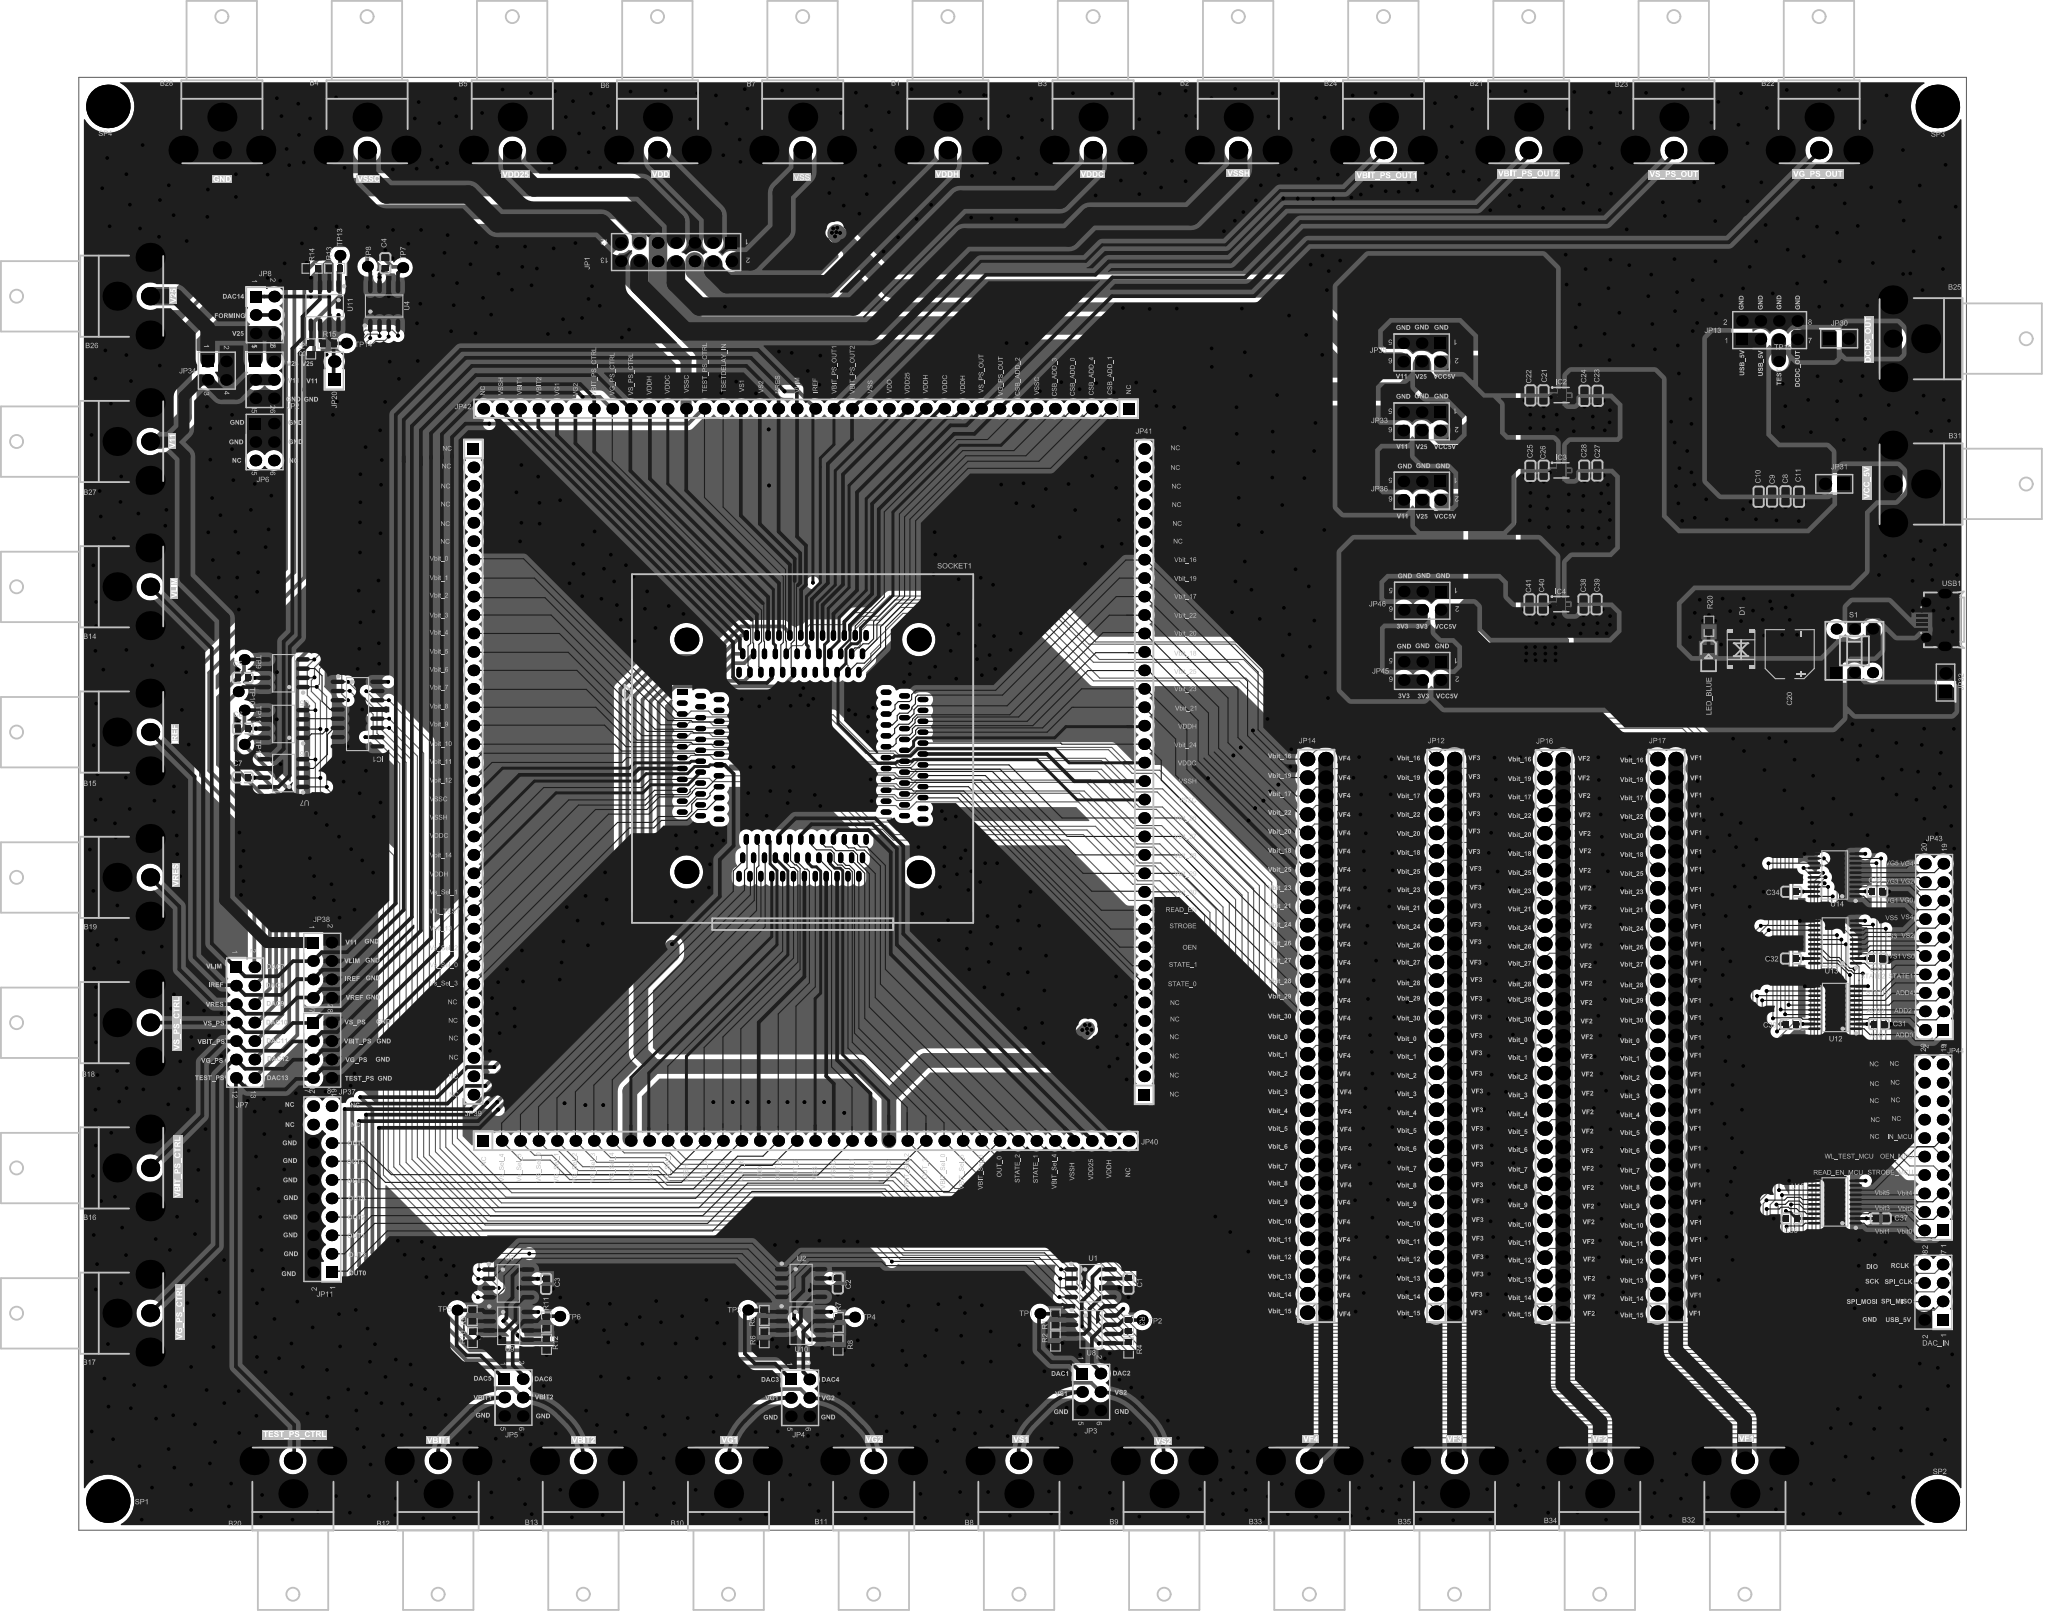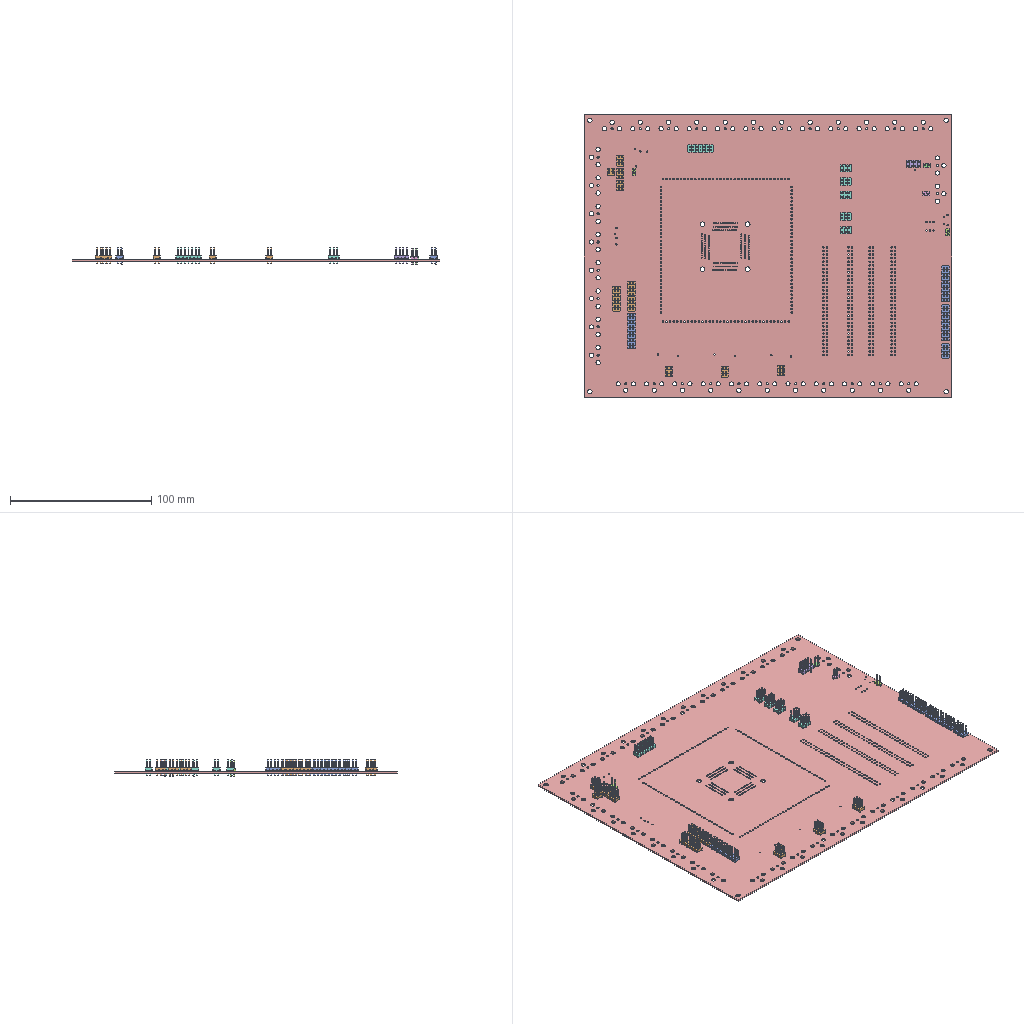Circuit board layout | Altium Designer | box 260 x 200 x 12.2 mm
Layer stack:
# Altium Designer layer stack of  (unit mm; dielectric type: 0 none, 1 core, 2 prepreg, 3 surface material)
index,name,kind,layer,copper_thickness_mm,dielectric_type,dielectric_thickness_mm,dielectric_material,dielectric_constant
0,Top Paste,other,,,,,,
1,Top Overlay,other,,,,,,
2,Top Solder,dielectric,,,3,0.0102,Solder Resist,3.5
3,Top Layer,copper,Top Layer,0.0356,,,,
4,Dielectric1,dielectric,,,1,0.32,FR-4,4.8
5,GND,copper,GND,0.0356,,,,
6,Dielectric3,dielectric,,,2,0.32,FR-4,4.8
7,POWER,copper,POWER,0.0356,,,,
8,Dielectric2,dielectric,,,1,0.32,FR-4,4.8
9,Bottom Layer,copper,Bottom Layer,0.0356,,,,
10,Bottom Solder,dielectric,,,3,0.0102,Solder Resist,3.5
11,Bottom Overlay,other,,,,,,
12,Bottom Paste,other,,,,,,
# drill layer pairs: low layer,high layer
drill_pair,Top Layer,Bottom Layer
Part placement:
Designator,Comment,Layer,Footprint,Center-X(mm),Center-Y(mm),Rotation
U15,TXS0108E,TopLayer,TSSOP-20_L6.5-W4.4-P0.65-LS6.4-BL,241.884,45.187,180
U14,TXS0108E,TopLayer,TSSOP-20_L6.5-W4.4-P0.65-LS6.4-BL,241.859,90.196,180
U13,TXS0108E,TopLayer,TSSOP-20_L6.5-W4.4-P0.65-LS6.4-BL,241.91,80.975,180
U12,TXS0108E,TopLayer,TSSOP-20_L6.5-W4.4-P0.65-LS6.4-BL,241.935,71.958,180
C37,100nF,TopLayer,0603C,248.209,42.926,360
C36,100nF,TopLayer,0603C,235.915,42.901,360
C35,100nF,TopLayer,0603C,247.726,87.91,360
C34,100nF,TopLayer,0603C,235.89,87.884,360
C33,100nF,TopLayer,0603C,247.726,78.689,360
C32,100nF,TopLayer,0603C,235.839,78.689,360
C31,100nF,TopLayer,0603C,247.955,69.672,360
C30,100nF,TopLayer,0603C,235.788,69.672,360
C20,100uF/25V,TopLayer,EC-D6.3x7.7,235.661,120.599,90
DAC_IN,DAC_IN,TopLayer,HDR2.54-LI-2x4P,255.448,32.766,90
U11,LM358,TopLayer,SO-8,33.866,168.564,270
U10,LM358,TopLayer,SO-8,99.469,28.16,360
U9,LM358,TopLayer,SO-8,59.21,28.135,360
U8,LM358,TopLayer,SO-8,139.424,27.652,360
U7,LTC1446,TopLayer,SO-8,28.208,104.228,180
U6,LTC1446,TopLayer,SO-8,28.208,110.984,180
U5,LTC1446,TopLayer,SO-8,28.208,117.969,180
U4,LTC1446,TopLayer,SO-8,42.055,168.519,90
U3,LTC1446,TopLayer,SO-8,59.16,33.977,360
U2,LTC1446,TopLayer,SO-8,99.495,34.028,360
U1,LTC1446,TopLayer,SO-8,139.373,34.002,360
D1,SMBJ5.0CA,TopLayer,SMB,228.956,121.209,90
LED_BLUE,LED,TopLayer,LED0805-R-RD,224.485,120.243,270
JP32,HEADER 1X2,TopLayer,HDR2.54-LI-2P,257.124,116.688,90
JP31,HEADER 1X2,TopLayer,HDR2.54-LI-2P,241.79,144.043,180
JP20,HEADER 1X2,TopLayer,HDR2.54-LI-2P,35.179,159.614,90
SP4,M3,TopLayer,M3,4,196,0
SP3,M3,TopLayer,M3,256,196,0
SP2,M3,TopLayer,M3,256,4,0
SP1,M3,TopLayer,M3,4,4,0
B1,bnc,TopLayer,BNC-TH_DOSIN-801-0072,119.706,192.246,360
B2,bnc,TopLayer,BNC-TH_DOSIN-801-0072,159.706,192.246,360
B3,bnc,TopLayer,BNC-TH_DOSIN-801-0072,139.706,192.246,360
B4,bnc,TopLayer,BNC-TH_DOSIN-801-0072,39.706,192.246,360
B5,bnc,TopLayer,BNC-TH_DOSIN-801-0072,59.706,192.246,360
B6,bnc,TopLayer,BNC-TH_DOSIN-801-0072,79.706,192.246,360
B7,bnc,TopLayer,BNC-TH_DOSIN-801-0072,99.706,192.246,360
B8,bnc,TopLayer,BNC-TH_DOSIN-801-0072,129.489,7.305,180
B9,bnc,TopLayer,BNC-TH_DOSIN-801-0072,149.489,7.305,180
B10,bnc,TopLayer,BNC-TH_DOSIN-801-0072,89.489,7.305,180
B11,bnc,TopLayer,BNC-TH_DOSIN-801-0072,109.489,7.305,180
B12,bnc,TopLayer,BNC-TH_DOSIN-801-0072,49.489,7.305,180
B13,bnc,TopLayer,BNC-TH_DOSIN-801-0072,69.489,7.305,180
B14,bnc,TopLayer,BNC-TH_DOSIN-801-0072,7.549,129.873,90
B15,bnc,TopLayer,BNC-TH_DOSIN-801-0072,7.549,109.873,90
B16,bnc,TopLayer,BNC-TH_DOSIN-801-0072,7.549,49.873,90
B17,bnc,TopLayer,BNC-TH_DOSIN-801-0072,7.549,29.873,90
B18,bnc,TopLayer,BNC-TH_DOSIN-801-0072,7.549,69.873,90
B19,bnc,TopLayer,BNC-TH_DOSIN-801-0072,7.549,89.873,90
B20,bnc,TopLayer,BNC-TH_DOSIN-801-0072,29.489,7.305,180
B21,bnc,TopLayer,BNC-TH_DOSIN-801-0072,199.706,192.246,360
B22,bnc,TopLayer,BNC-TH_DOSIN-801-0072,239.706,192.246,360
B23,bnc,TopLayer,BNC-TH_DOSIN-801-0072,219.706,192.246,360
B24,bnc,TopLayer,BNC-TH_DOSIN-801-0072,179.706,192.246,360
B25,bnc,TopLayer,BNC-TH_DOSIN-801-0072,252.113,164.017,270
B26,bnc,TopLayer,BNC-TH_DOSIN-801-0072,7.549,169.873,90
B27,bnc,TopLayer,BNC-TH_DOSIN-801-0072,7.549,149.873,90
B28,bnc,TopLayer,BNC-TH_DOSIN-801-0072,19.706,192.246,360
B31,bnc,TopLayer,BNC-TH_DOSIN-801-0072,252.113,144.017,270
B32,bnc,TopLayer,BNC-TH_DOSIN-801-0072,229.489,7.305,180
B33,bnc,TopLayer,BNC-TH_DOSIN-801-0072,169.489,7.305,180
B34,bnc,TopLayer,BNC-TH_DOSIN-801-0072,209.489,7.305,180
B35,bnc,TopLayer,BNC-TH_DOSIN-801-0072,189.489,7.305,180
IC1,74HC595,TopLayer,SOIC-16_L9.9-W3.9-P1.27-LS6.0-BL,38.396,112.346,270
IC2,TPS74511PQWDRVRQ1,TopLayer,WSON-6_L2.0-W2.0-P0.65-BL-EP,204.241,156.261,270
IC3,TPS74525PQWDRVRQ1,TopLayer,WSON-6_L2.0-W2.0-P0.65-BL-EP,204.216,145.898,270
IC4,TPS74533PQWDRVRQ1,TopLayer,WSON-6_L2.0-W2.0-P0.65-BL-EP,204.191,127.483,270
S1,TK-6700-1,TopLayer,SW-TH_6P-L8.0-W8.0-P2.50,244.57,121.053,360
SOCKET1,M189,TopLayer,YAMAICHI_IC51-1444-1354-7,99.695,106.604,360
USB1,MICROXNJ,TopLayer,MICRO-USB-SMD_MICROXNJ,255.46,125.295,90
C1,104,TopLayer,0603C,144.58,33.951,90
C2,104,TopLayer,0603C,104.549,33.977,90
C3,104,TopLayer,0603C,64.367,33.926,90
C4,104,TopLayer,0603C,42.215,174.396,270
C5,104,TopLayer,0603C,22.569,117.334,360
C6,104,TopLayer,0603C,22.62,110.349,360
C7,104,TopLayer,0603C,22.569,103.618,360
C8,104,TopLayer,0603C,235.084,142.315,270
C9,104,TopLayer,0603C,233.23,142.29,270
C10,104,TopLayer,0603C,231.376,142.265,270
C11,104,TopLayer,0603C,236.939,142.265,270
C21,100nF,TopLayer,0603C,201.741,156.21,270
C22,10uF/16V,TopLayer,0603C,199.938,156.21,270
C23,100nF,TopLayer,0603C,209.209,156.16,270
C24,10uF/16V,TopLayer,0603C,207.38,156.16,270
C25,100nF,TopLayer,0603C,199.938,145.822,270
C26,10nF/16V,TopLayer,0603C,201.766,145.847,270
C27,100nF,TopLayer,0603C,209.158,145.873,270
C28,10nF/16V,TopLayer,0603C,207.354,145.847,270
C38,10nF/16V,TopLayer,0603C,207.253,127.432,270
C39,100nF,TopLayer,0603C,209.056,127.458,270
C40,10nF/16V,TopLayer,0603C,201.665,127.432,270
C41,100nF,TopLayer,0603C,199.811,127.432,270
R1,1k,TopLayer,0603R,134.521,29.049,90
R2,1k,TopLayer,0603R,134.521,26.052,270
R3,1k,TopLayer,0603R,144.605,28.186,270
R4,1k,TopLayer,0603R,144.602,25.095,270
R5,1k,TopLayer,0603R,94.415,29.557,90
R6,1k,TopLayer,0603R,94.415,26.509,270
R7,1k,TopLayer,0603R,104.626,28.592,270
R8,1k,TopLayer,0603R,104.597,25.502,270
R9,1k,TopLayer,0603R,54.207,29.557,90
R10,1k,TopLayer,0603R,54.232,26.535,270
R11,1k,TopLayer,0603R,64.392,28.643,270
R12,1k,TopLayer,0603R,64.44,25.603,270
R13,1k,TopLayer,0603R,35.237,173.72,360
R14,1k,TopLayer,0603R,32.138,173.695,180
R15,1k,TopLayer,0603R,34.348,163.382,180
R16,1k,TopLayer,0603R,31.961,162.62,270
R20,1k,TopLayer,0603R,224.536,124.435,90
TP1,OUT1,TopLayer,TP1.0,132.388,29.811,360
TP2,OUT2,TopLayer,TP1.0,146.459,28.922,90
TP3,OUT3,TopLayer,TP1.0,92.154,30.319,90
TP4,OUT4,TopLayer,TP1.0,106.861,29.329,90
TP5,OUT5,TopLayer,TP1.0,52.098,30.294,90
TP6,OUT6,TopLayer,TP1.0,66.243,29.439,90
TP7,OUT7,TopLayer,TP1.0,44.62,173.803,180
TP8,OUT8,TopLayer,TP1.0,39.751,173.965,180
TP9,OUT9,TopLayer,TP1.0,22.797,119.849,360
TP10,OUT10,TopLayer,TP1.0,21.959,115.429,360
TP11,OUT11,TopLayer,TP1.0,22.797,112.889,360
TP12,OUT12,TopLayer,TP1.0,22.79,108.181,360
TP13,OUT13,TopLayer,TP1.0,35.966,175.489,360
TP14,OUT14,TopLayer,TP1.0,36.855,163.398,360
TP15,3V3,TopLayer,TP1.0,234.137,160.909,90
JP1,HEADER 7X2,TopLayer,HDR2.54-LI-2x7P,82.271,175.946,180
JP2,HEADER 3X2,TopLayer,HDR2.54-LI-2x3P,25.594,158.357,270
JP8,HEADER 3X2,TopLayer,HDR2.54-LI-2x3P,25.629,167.285,270
JP11,HEADER 10X2,TopLayer,HDR2.54-LI-2x10P,33.544,46.942,90
JP13,HEADER 4X2,TopLayer,HDR2.54-LI-2x4P,232.893,165.202,360
JP33,HEADER 3X2,TopLayer,HDR2.54-LI-2x3P,184.963,152.64,180
JP35,HEADER 3X2,TopLayer,HDR2.54-LI-2x3P,184.963,162.129,180
JP36,HEADER 3X2,TopLayer,HDR2.54-LI-2x3P,184.988,143.104,180
JP37,HEADER 4X2,TopLayer,HDR2.54-LI-2x4P,33.526,66.068,270
JP38,HEADER 4X2,TopLayer,HDR2.54-LI-2x4P,33.526,77.091,270
JP43,HEADER 10X2,TopLayer,HDR2.54-LI-2x10P,255.549,80.315,90
JP44,HEADER 10X2,TopLayer,HDR2.54-LI-2x10P,255.448,52.705,90
JP45,HEADER 3X2,TopLayer,HDR2.54-LI-2x3P,185.039,118.288,180
JP46,HEADER 3X2,TopLayer,HDR2.54-LI-2x3P,185.039,127.951,180
JP3,HEADER 3X2,TopLayer,HDR2.54-LI-2x3P,139.451,19.025,270
JP4,HEADER 3X2,TopLayer,HDR2.54-LI-2x3P,99.352,18.221,270
JP5,HEADER 3X2,TopLayer,HDR2.54-LI-2x3P,59.873,18.263,270
JP6,HEADER 2X2,TopLayer,HDR2.54-LI-2x3P,25.594,149.797,270
JP7,HEADER 7X2,TopLayer,HDR2.54-LI-2x7P,22.911,69.875,270
JP34,HEADER 2X2,TopLayer,HDR2.54-LI-2x2P,19.015,159.627,270
JP12,HEADER 31X2,TopLayer,HDR2.54-LI-2x31P,188.214,68.047,90
JP14,HEADER 31X2,TopLayer,HDR2.54-LI-2x31P,170.459,68.047,90
JP16,HEADER 31X2,TopLayer,HDR2.54-LI-2x31P,203.149,67.996,90
JP17,HEADER 31X2,TopLayer,HDR2.54-LI-2x31P,218.694,68.047,90
JP30,HEADER 1X2,TopLayer,HDR2.54-LI-2P,242.468,164.033,360
JP39,HEADER 36X1,TopLayer,HDR2.54-LI-1x36P,54.356,104.394,270
JP40,HEADER  36X1,TopLayer,HDR2.54-LI-1x36P,100.152,53.594,360
JP41,HEADER  36X1,TopLayer,HDR2.54-LI-1x36P,146.736,104.394,90
JP42,HEADER  36X1,TopLayer,HDR2.54-LI-1x36P,100.152,154.382,180
Pad and via stacks:
# Altium Designer via and pad stacks of  (unit mm). Each distinct definition once, with the count of objects using it.
# via: kind,start_layer,end_layer,hole_mm,diameter_mm,mode(0 simple;1 top-mid-bottom;2 full stack),diameter_per_layer,count,example_net
# pad: kind,layer,hole_mm,hole_type(0 round;1 square;2 slot),plating,top_size,top_shape(1 round;2 rect;3 octagon;9 rounded rect),mid_size,bottom_size,mode,footprint,size_per_layer,count,example
pad,Multi-Layer,3.2,0,plated,6x6,1,6x6,6x6,0,M3,,4,SP1.1
pad,Multi-Layer,3,0,plated,4x4,1,4x4,4x4,0,BNC-TH_DOSIN-801-0072,,99,B35.4
pad,Multi-Layer,1.5,0,plated,2.5x2.5,1,2.5x2.5,2.5x2.5,0,BNC-TH_DOSIN-801-0072,,33,B35.1
pad,Multi-Layer,1.1,0,plated,1.6x1.6,2,1.6x1.6,1.6x1.6,0,HDR2.54-LI-1x36P,,4,JP39.1
pad,Multi-Layer,1.1,0,plated,1.6x1.6,1,1.6x1.6,1.6x1.6,0,HDR2.54-LI-1x36P,,140,JP39.2
pad,Multi-Layer,1.02,0,plated,2x2,1,2x2,2x2,0,HDR2.54-LI-2x31P,,248,JP12.1
pad,Multi-Layer,0.9,0,plated,1.6x1.6,2,1.6x1.6,1.6x1.6,0,HDR2.54-LI-2x2P,,1,JP34.1
pad,Multi-Layer,0.9,0,plated,1.6x1.6,1,1.6x1.6,1.6x1.6,0,HDR2.54-LI-2x2P,,3,JP34.2
pad,Multi-Layer,0.9,0,plated,1.6x1.6,1,1.6x1.6,1.6x1.6,0,HDR2.54-LI-2x10P,,57,JP11.20
pad,Multi-Layer,0.9,0,plated,1.6x1.6,2,1.6x1.6,1.6x1.6,0,HDR2.54-LI-2x10P,,3,JP11.1
pad,Multi-Layer,0.9,0,plated,1.6x1.6,1,1.6x1.6,1.6x1.6,0,HDR2.54-LI-2x3P,,55,JP2.6
pad,Multi-Layer,0.9,0,plated,1.6x1.6,2,1.6x1.6,1.6x1.6,0,HDR2.54-LI-2x3P,,11,JP2.1
pad,Multi-Layer,0.9,0,plated,1.6x1.6,2,1.6x1.6,1.6x1.6,0,HDR2.54-LI-2x7P,,2,JP1.1
pad,Multi-Layer,0.9,0,plated,1.6x1.6,1,1.6x1.6,1.6x1.6,0,HDR2.54-LI-2x7P,,26,JP1.2
pad,Multi-Layer,1,0,plated,1.5x1.5,1,1.5x1.5,1.5x1.5,0,TP1.0,,15,TP1.1
pad,Multi-Layer,0.7,0,plated,1.3x1.3,1,1.3x1.3,1.3x1.3,0,MICRO-USB-SMD_MICROXNJ,,2,USB1.6
pad,Multi-Layer,0.7,2,plated,1.3x1.8,1,1.3x1.8,1.3x1.8,0,MICRO-USB-SMD_MICROXNJ,,2,USB1.8
pad,Multi-Layer,1,0,plated,1.524x1.524,1,1.524x1.524,1.524x1.524,0,SW-TH_6P-L8.0-W8.0-P2.50,,5,S1.4
pad,Multi-Layer,1,0,plated,1.524x1.524,2,1.524x1.524,1.524x1.524,0,SW-TH_6P-L8.0-W8.0-P2.50,,1,S1.1
pad,Multi-Layer,0.9,0,plated,1.7x1.7,1,1.7x1.7,1.7x1.7,0,HDR2.54-LI-2P,,4,JP32.2
pad,Multi-Layer,0.9,0,plated,1.7x1.7,2,1.7x1.7,1.7x1.7,0,HDR2.54-LI-2P,,4,JP32.1
pad,Multi-Layer,0.9,0,plated,1.6x1.6,2,1.6x1.6,1.6x1.6,0,HDR2.54-LI-2x4P,,4,DAC_IN.1
pad,Multi-Layer,0.9,0,plated,1.6x1.6,1,1.6x1.6,1.6x1.6,0,HDR2.54-LI-2x4P,,28,DAC_IN.2
pad,Multi-Layer,0.65,0,plated,1.5x0.73,2,1.5x0.73,1.5x0.73,0,YAMAICHI_IC51-1444-1354-7,,1,SOCKET1.1
pad,Multi-Layer,0.65,0,plated,1.5x0.73,1,1.5x0.73,1.5x0.73,0,YAMAICHI_IC51-1444-1354-7,,71,SOCKET1.2
pad,Multi-Layer,0.65,0,plated,0.73x1.5,1,0.73x1.5,0.73x1.5,0,YAMAICHI_IC51-1444-1354-7,,72,SOCKET1.37
pad,Multi-Layer,3.3,0,unplated,3.3x3.3,1,3.3x3.3,3.3x3.3,0,YAMAICHI_IC51-1444-1354-7,,4,SOCKET1.
pad,Top Layer,0,0,plated,0.8065x0.864,2,0.8065x0.864,0.8065x0.864,0,0603R,,34,R1.1
pad,Top Layer,0,0,plated,1.6x0.4,2,1.6x0.4,1.6x0.4,0,MICRO-USB-SMD_MICROXNJ,,5,USB1.1
pad,Top Layer,0,0,plated,1x1.6,2,1x1.6,1x1.6,0,WSON-6_L2.0-W2.0-P0.65-BL-EP,,3,IC2.7
pad,Top Layer,0,0,plated,0.4x0.45,2,0.4x0.45,0.4x0.45,0,WSON-6_L2.0-W2.0-P0.65-BL-EP,,18,IC2.6
pad,Top Layer,0,0,plated,0.602x1.971,1,0.602x1.971,0.602x1.971,0,SOIC-16_L9.9-W3.9-P1.27-LS6.0-BL,,16,IC1.9
pad,Top Layer,0,0,plated,1x1.399,2,1x1.399,1x1.399,0,LED0805-R-RD,,2,LED_BLUE.2
pad,Top Layer,0,0,plated,2.047x2.241,2,2.047x2.241,2.047x2.241,0,SMB,,2,D1.1
pad,Top Layer,0,0,plated,0.63x1.865,1,0.63x1.865,0.63x1.865,0,SO-8,,88,U11.5
pad,Top Layer,0,0,plated,3.5x1.2,2,3.5x1.2,3.5x1.2,0,EC-D6.3x7.7,,2,C20.2
pad,Top Layer,0,0,plated,0.8x0.9,2,0.8x0.9,0.8x0.9,0,0603C,,62,C37.2
pad,Top Layer,0,0,plated,0.364x1.742,1,0.364x1.742,0.364x1.742,0,TSSOP-20_L6.5-W4.4-P0.65-LS6.4-BL,,80,U15.1
via,Top Layer,Bottom Layer,0.3048,0.508,0,,1759,VCC_5V
Copper pours:
name,layer,net,type(0 solid;1 hatched;2 none)
Bottom Layer-No Net,Top Layer,NetB25_1,0
Bottom Layer-No Net,Top Layer,DCDC_OUT,0
Bottom Layer-No Net,Top Layer,USB_5V,0
Bottom Layer-No Net,Top Layer,3V3,0
Bottom Layer-No Net,Top Layer,V11,0
Bottom Layer-No Net,Top Layer,V25,0
Bottom Layer-No Net,Top Layer,VCC_5V,0
Bottom Layer-No Net,Top Layer,NetJP32_1,0
Bottom Layer-No Net,Top Layer,NetS1_5,0
Bottom Layer-No Net,Top Layer,GND,0
Bottom Layer-No Net,Bottom Layer,VCC_5V,0
Bottom Layer-No Net,Bottom Layer,GND,0
Bottom Layer-No Net,POWER,GND,0
Design rules, without the lines most boards share:
# Altium Designer design rules of  (exported by Altium Designer, unit mm)
# columns: name | kind | enabled | priority | scope1 | scope2 | descriptor | typed fields (field=value)
Clearance | 0 | enabled | 2 | All | All | Clearance Constraint (Gap=6mil) (All),(All) | gap=0.1524
PlaneConnect | 6 | enabled | 1 | All | All | Power Plane Connect Rule(Direct Connect )(Expansion=20mil) (Conductor Width=10mil) (Air Gap=10mil) (Entries=4) (All) | relief_conductor_width=0.254 relief_entries=4 relief_expansion=0.508
PlaneClearance | 12 | enabled | 1 | All | All | Power Plane Clearance (Clearance =6mil) (All) | clearance=0.1524
PolygonConnect | 20 | enabled | 1 | All | All | Polygon Connect Rule(Direct Connect )(Conductor Width=10mil) (Relief Angle=90 Angle) (Entries=4) (Air Gap Width=10mil) (All),(All) | connect_style(0=relief,1=direct,2=none)=1 relief_conductor_width=0.254 relief_entries=4
Width | 2 | enabled | 1 | All | All | Width Constraint (Min=6mil) (Max=200mil) (Preferred=10mil) (All) |
RoutingVias | 11 | enabled | 1 | All | All | Routing Via (MinHoleWidth=12mil) (MaxHoleWidth=12mil) (PreferredHoleWidth=12mil) (MinWidth=20mil) (MaxWidth=20mil) (PreferedWidth=20mil) (All) | via_min_hole=0.3048 via_max_hole=0.3048 via_preferred_diameter=0.508 via_preferred_hole=0.3048
SolderMaskExpansion | 13 | enabled | 1 | All | All | Solder Mask Expansion (Expansion =4mil) (All) | expansion=0.1016
HoleSize | 42 | enabled | 1 | All | All | Hole Size Constraint (Min=1mil) (Max=500mil) (All) |
DiffPairsRouting | 51 | enabled | 1 | All | All | Differential Pairs Uncoupled Length using the Gap Constraints (Min=6mil) (Max=10mil) (Prefered=10mil)  and Width Constraints (Min=15mil) (Max=15mil) (Prefered=15mil) (All) |
HoleToHoleClearance | 52 | enabled | 1 | All | All | Hole To Hole Clearance (Gap=0mil) (All),(All) | gap=0
MinimumSolderMaskSliver | 53 | enabled | 1 | All | All | Minimum Solder Mask Sliver (Gap=0mil) (All),(All) |
SilkscreenOverComponentPads | 54 | enabled | 1 | IsPad | All | Silk To Solder Mask (Clearance=0mil) (IsPad),(All) |
SilkToSilkClearance | 55 | enabled | 1 | All | All | Silk to Silk (Clearance=0mil) (All),(All) |
Clearance_1 | 0 | enabled | 1 | inpolygon | All | Clearance Constraint (Gap=6mil) (inpolygon),(All) | gap=0.1524
Classes set for this board:
# Altium Designer classes of  (member kind: 0 net, 1 component, 2 from-to, 3 pad, 4 layer, 5 differential pair, 6 design channel, 7 polygon, 8 structure, 9 xSignal)
# columns: class name | member kind | superclass | members
PCB2 | 1 | no | C20; C21; C22; C23; C24; C25; C26; C27; C28; C30; C31; C32; C33; C34; C35; C36; C37; C38; C39; C40; C41; D1; JP1; JP2; JP3; JP4; JP5; JP6; JP7; JP8; JP11; JP12; JP13; JP14; JP16; JP17; JP30; JP32; JP33; JP34; JP35; JP36; JP37; JP38; JP39; JP40; JP41; JP42; JP43; JP44; JP45; JP46; LED_BLUE; R20; SP1; SP2; SP3; SP4; TP15; U12; U13; U14; U15; B1; B2; B3; B4; B5; B6; B7; B8; B9; B10; B11; B12; B13; B14; B15; B16; B17; B18; B19; B20; B21; B22; B23; B24; B25; B26; B27; B28; B32; B33; B34; B35; C21; C22; C23; C24; C25; C26; C27; C28; C38; C39; C40; C41; IC2; IC3; IC4; S1; SOCKET1; USB1; R20; TP15; JP1; JP2; JP8; JP11; JP13; JP33; JP35; JP36; JP37; JP38; JP43; JP44; JP45; JP46; JP3; JP4; JP5; JP6; JP7; JP34; JP12; JP14; JP16; JP17; JP30; JP39; JP40; JP41; JP42; SP1; SP2; SP3; SP4; JP32; LED_BLUE; D1; C20; C30; C31; C32; C33; C34; C35; C36; C37; U12; U13; U14; U15;
DacModule | 1 | no | B31; C1; C2; C3; C4; C5; C6; C7; C8; C9; C10; C11; DAC_IN; IC1; JP20; JP31; R1; R2; R3; R4; R5; R6; R7; R8; R9; R10; R11; R12; R13; R14; R15; R16; TP1; TP2; TP3; TP4; TP5; TP6; TP7; TP8; TP9; TP10; TP11; TP12; TP13; TP14; U1; U2; U3; U4; U5; U6; U7; U8; U9; U10; U11;